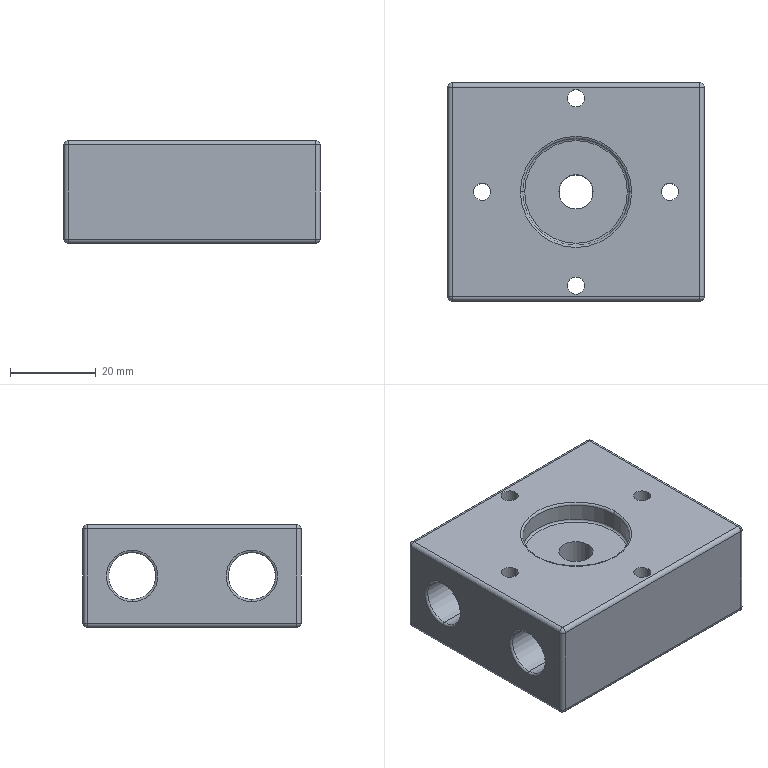Part | SolidWorks | features ICE 3, Fillet 2, Cut 1, Extrusion 1 | 1 solid | 55 faces | box 60 x 51 x 24 mm | volume 57298 mm3 | cylinder 28 | torus 12 | sphere 8 | plane 7 | commonest cylinder face diameters 2 x12 4 x8 11 x4 8 x2 25 x2
STEP:
#1=CARTESIAN_POINT('',(-19.92,0.,12.));
#2=VERTEX_POINT('',#1);
#3=CARTESIAN_POINT('',(-23.92,0.,12.));
#4=VERTEX_POINT('',#3);
#5=CARTESIAN_POINT('',(-21.92,0.,12.));
#6=DIRECTION('',(0.,0.,-1.));
#7=DIRECTION('',(-1.,0.,0.));
#8=AXIS2_PLACEMENT_3D('',#5,#6,#7);
#9=CIRCLE('',#8,2.);
#10=EDGE_CURVE('',#2,#4,#9,.T.);
#11=ORIENTED_EDGE('',*,*,#10,.F.);
#12=CARTESIAN_POINT('',(-19.92,0.,-12.));
#13=VERTEX_POINT('',#12);
#14=CARTESIAN_POINT('',(-19.92,0.,12.));
#15=DIRECTION('',(0.,0.,-1.));
#16=VECTOR('',#15,1000.);
#17=LINE('',#14,#16);
#18=EDGE_CURVE('',#2,#13,#17,.T.);
#19=ORIENTED_EDGE('',*,*,#18,.T.);
#20=CARTESIAN_POINT('',(-23.92,0.,-12.));
#21=VERTEX_POINT('',#20);
#22=CARTESIAN_POINT('',(-21.92,0.,-12.));
#23=DIRECTION('',(0.,0.,-1.));
#24=DIRECTION('',(-1.,0.,0.));
#25=AXIS2_PLACEMENT_3D('',#22,#23,#24);
#26=CIRCLE('',#25,2.);
#27=EDGE_CURVE('',#13,#21,#26,.T.);
#28=ORIENTED_EDGE('',*,*,#27,.T.);
#29=CARTESIAN_POINT('',(-23.92,0.,12.));
#30=DIRECTION('',(0.,0.,-1.));
#31=VECTOR('',#30,1000.);
#32=LINE('',#29,#31);
#33=EDGE_CURVE('',#4,#21,#32,.T.);
#34=ORIENTED_EDGE('',*,*,#33,.F.);
#35=EDGE_LOOP('',(#11,#19,#28,#34));
#36=FACE_OUTER_BOUND('',#35,.T.);
#37=CARTESIAN_POINT('',(-21.92,0.,12.));
#38=DIRECTION('',(0.,0.,-1.));
#39=DIRECTION('',(-1.,0.,0.));
#40=AXIS2_PLACEMENT_3D('',#37,#38,#39);
#41=CYLINDRICAL_SURFACE('',#40,2.);
#42=ADVANCED_FACE('',(#36),#41,.F.);
#43=CARTESIAN_POINT('',(2.,21.92,12.));
#44=VERTEX_POINT('',#43);
#45=CARTESIAN_POINT('',(-2.,21.92,12.));
#46=VERTEX_POINT('',#45);
#47=CARTESIAN_POINT('',(0.,21.92,12.));
#48=DIRECTION('',(0.,0.,-1.));
#49=DIRECTION('',(-1.,0.,0.));
#50=AXIS2_PLACEMENT_3D('',#47,#48,#49);
#51=CIRCLE('',#50,2.);
#52=EDGE_CURVE('',#44,#46,#51,.T.);
#53=ORIENTED_EDGE('',*,*,#52,.F.);
#54=CARTESIAN_POINT('',(2.,21.92,-12.));
#55=VERTEX_POINT('',#54);
#56=CARTESIAN_POINT('',(2.,21.92,12.));
#57=DIRECTION('',(0.,0.,-1.));
#58=VECTOR('',#57,1000.);
#59=LINE('',#56,#58);
#60=EDGE_CURVE('',#44,#55,#59,.T.);
#61=ORIENTED_EDGE('',*,*,#60,.T.);
#62=CARTESIAN_POINT('',(-2.,21.92,-12.));
#63=VERTEX_POINT('',#62);
#64=CARTESIAN_POINT('',(0.,21.92,-12.));
#65=DIRECTION('',(0.,0.,-1.));
#66=DIRECTION('',(-1.,0.,0.));
#67=AXIS2_PLACEMENT_3D('',#64,#65,#66);
#68=CIRCLE('',#67,2.);
#69=EDGE_CURVE('',#55,#63,#68,.T.);
#70=ORIENTED_EDGE('',*,*,#69,.T.);
#71=CARTESIAN_POINT('',(-2.,21.92,12.));
#72=DIRECTION('',(0.,0.,-1.));
#73=VECTOR('',#72,1000.);
#74=LINE('',#71,#73);
#75=EDGE_CURVE('',#46,#63,#74,.T.);
#76=ORIENTED_EDGE('',*,*,#75,.F.);
#77=EDGE_LOOP('',(#53,#61,#70,#76));
#78=FACE_OUTER_BOUND('',#77,.T.);
#79=CARTESIAN_POINT('',(0.,21.92,12.));
#80=DIRECTION('',(0.,0.,-1.));
#81=DIRECTION('',(-1.,0.,0.));
#82=AXIS2_PLACEMENT_3D('',#79,#80,#81);
#83=CYLINDRICAL_SURFACE('',#82,2.);
#84=ADVANCED_FACE('',(#78),#83,.F.);
#85=CARTESIAN_POINT('',(23.92,0.,12.));
#86=VERTEX_POINT('',#85);
#87=CARTESIAN_POINT('',(19.92,0.,12.));
#88=VERTEX_POINT('',#87);
#89=CARTESIAN_POINT('',(21.92,0.,12.));
#90=DIRECTION('',(0.,0.,-1.));
#91=DIRECTION('',(-1.,0.,0.));
#92=AXIS2_PLACEMENT_3D('',#89,#90,#91);
#93=CIRCLE('',#92,2.);
#94=EDGE_CURVE('',#86,#88,#93,.T.);
#95=ORIENTED_EDGE('',*,*,#94,.F.);
#96=CARTESIAN_POINT('',(23.92,0.,-12.));
#97=VERTEX_POINT('',#96);
#98=CARTESIAN_POINT('',(23.92,0.,12.));
#99=DIRECTION('',(0.,0.,-1.));
#100=VECTOR('',#99,1000.);
#101=LINE('',#98,#100);
#102=EDGE_CURVE('',#86,#97,#101,.T.);
#103=ORIENTED_EDGE('',*,*,#102,.T.);
#104=CARTESIAN_POINT('',(19.92,0.,-12.));
#105=VERTEX_POINT('',#104);
#106=CARTESIAN_POINT('',(21.92,0.,-12.));
#107=DIRECTION('',(0.,0.,-1.));
#108=DIRECTION('',(-1.,0.,0.));
#109=AXIS2_PLACEMENT_3D('',#106,#107,#108);
#110=CIRCLE('',#109,2.);
#111=EDGE_CURVE('',#97,#105,#110,.T.);
#112=ORIENTED_EDGE('',*,*,#111,.T.);
#113=CARTESIAN_POINT('',(19.92,0.,12.));
#114=DIRECTION('',(0.,0.,-1.));
#115=VECTOR('',#114,1000.);
#116=LINE('',#113,#115);
#117=EDGE_CURVE('',#88,#105,#116,.T.);
#118=ORIENTED_EDGE('',*,*,#117,.F.);
#119=EDGE_LOOP('',(#95,#103,#112,#118));
#120=FACE_OUTER_BOUND('',#119,.T.);
#121=CARTESIAN_POINT('',(21.92,0.,12.));
#122=DIRECTION('',(0.,0.,-1.));
#123=DIRECTION('',(-1.,0.,0.));
#124=AXIS2_PLACEMENT_3D('',#121,#122,#123);
#125=CYLINDRICAL_SURFACE('',#124,2.);
#126=ADVANCED_FACE('',(#120),#125,.F.);
#127=CARTESIAN_POINT('',(2.,-21.92,12.));
#128=VERTEX_POINT('',#127);
#129=CARTESIAN_POINT('',(-2.,-21.92,12.));
#130=VERTEX_POINT('',#129);
#131=CARTESIAN_POINT('',(0.,-21.92,12.));
#132=DIRECTION('',(0.,0.,-1.));
#133=DIRECTION('',(-1.,0.,0.));
#134=AXIS2_PLACEMENT_3D('',#131,#132,#133);
#135=CIRCLE('',#134,2.);
#136=EDGE_CURVE('',#128,#130,#135,.T.);
#137=ORIENTED_EDGE('',*,*,#136,.F.);
#138=CARTESIAN_POINT('',(2.,-21.92,-12.));
#139=VERTEX_POINT('',#138);
#140=CARTESIAN_POINT('',(2.,-21.92,12.));
#141=DIRECTION('',(0.,0.,-1.));
#142=VECTOR('',#141,1000.);
#143=LINE('',#140,#142);
#144=EDGE_CURVE('',#128,#139,#143,.T.);
#145=ORIENTED_EDGE('',*,*,#144,.T.);
#146=CARTESIAN_POINT('',(-2.,-21.92,-12.));
#147=VERTEX_POINT('',#146);
#148=CARTESIAN_POINT('',(0.,-21.92,-12.));
#149=DIRECTION('',(0.,0.,-1.));
#150=DIRECTION('',(-1.,0.,0.));
#151=AXIS2_PLACEMENT_3D('',#148,#149,#150);
#152=CIRCLE('',#151,2.);
#153=EDGE_CURVE('',#139,#147,#152,.T.);
#154=ORIENTED_EDGE('',*,*,#153,.T.);
#155=CARTESIAN_POINT('',(-2.,-21.92,12.));
#156=DIRECTION('',(0.,0.,-1.));
#157=VECTOR('',#156,1000.);
#158=LINE('',#155,#157);
#159=EDGE_CURVE('',#130,#147,#158,.T.);
#160=ORIENTED_EDGE('',*,*,#159,.F.);
#161=EDGE_LOOP('',(#137,#145,#154,#160));
#162=FACE_OUTER_BOUND('',#161,.T.);
#163=CARTESIAN_POINT('',(0.,-21.92,12.));
#164=DIRECTION('',(0.,0.,-1.));
#165=DIRECTION('',(-1.,0.,0.));
#166=AXIS2_PLACEMENT_3D('',#163,#164,#165);
#167=CYLINDRICAL_SURFACE('',#166,2.);
#168=ADVANCED_FACE('',(#162),#167,.F.);
#169=CARTESIAN_POINT('',(-4.,0.,7.));
#170=VERTEX_POINT('',#169);
#171=CARTESIAN_POINT('',(4.,0.,7.));
#172=VERTEX_POINT('',#171);
#173=CARTESIAN_POINT('',(0.,0.,7.));
#174=DIRECTION('',(0.,0.,1.));
#175=DIRECTION('',(1.,0.,0.));
#176=AXIS2_PLACEMENT_3D('',#173,#174,#175);
#177=CIRCLE('',#176,4.);
#178=EDGE_CURVE('',#170,#172,#177,.T.);
#179=ORIENTED_EDGE('',*,*,#178,.T.);
#180=CARTESIAN_POINT('',(4.,0.,-12.));
#181=VERTEX_POINT('',#180);
#182=CARTESIAN_POINT('',(4.,0.,12.));
#183=DIRECTION('',(0.,0.,-1.));
#184=VECTOR('',#183,1000.);
#185=LINE('',#182,#184);
#186=EDGE_CURVE('',#172,#181,#185,.T.);
#187=ORIENTED_EDGE('',*,*,#186,.T.);
#188=CARTESIAN_POINT('',(-4.,0.,-12.));
#189=VERTEX_POINT('',#188);
#190=CARTESIAN_POINT('',(0.,0.,-12.));
#191=DIRECTION('',(0.,0.,-1.));
#192=DIRECTION('',(-1.,0.,0.));
#193=AXIS2_PLACEMENT_3D('',#190,#191,#192);
#194=CIRCLE('',#193,4.);
#195=EDGE_CURVE('',#181,#189,#194,.T.);
#196=ORIENTED_EDGE('',*,*,#195,.T.);
#197=CARTESIAN_POINT('',(-4.,0.,12.));
#198=DIRECTION('',(0.,0.,-1.));
#199=VECTOR('',#198,1000.);
#200=LINE('',#197,#199);
#201=EDGE_CURVE('',#170,#189,#200,.T.);
#202=ORIENTED_EDGE('',*,*,#201,.F.);
#203=EDGE_LOOP('',(#179,#187,#196,#202));
#204=FACE_OUTER_BOUND('',#203,.T.);
#205=CARTESIAN_POINT('',(0.,0.,12.));
#206=DIRECTION('',(0.,0.,-1.));
#207=DIRECTION('',(-1.,0.,0.));
#208=AXIS2_PLACEMENT_3D('',#205,#206,#207);
#209=CYLINDRICAL_SURFACE('',#208,4.);
#210=ADVANCED_FACE('',(#204),#209,.F.);
#211=CARTESIAN_POINT('',(-29.5,14.,5.5));
#212=VERTEX_POINT('',#211);
#213=CARTESIAN_POINT('',(-29.5,14.,-5.5));
#214=VERTEX_POINT('',#213);
#215=CARTESIAN_POINT('',(-29.5,14.,0.));
#216=DIRECTION('',(-1.,0.,0.));
#217=DIRECTION('',(0.,0.,-1.));
#218=AXIS2_PLACEMENT_3D('',#215,#216,#217);
#219=CIRCLE('',#218,5.5);
#220=EDGE_CURVE('',#212,#214,#219,.T.);
#221=ORIENTED_EDGE('',*,*,#220,.F.);
#222=CARTESIAN_POINT('',(-30.,14.,6.));
#223=VERTEX_POINT('',#222);
#224=CARTESIAN_POINT('',(-29.5,14.,6.));
#225=DIRECTION('',(0.,1.,0.));
#226=DIRECTION('',(0.,0.,1.));
#227=AXIS2_PLACEMENT_3D('',#224,#225,#226);
#228=CIRCLE('',#227,0.5);
#229=EDGE_CURVE('',#212,#223,#228,.T.);
#230=ORIENTED_EDGE('',*,*,#229,.T.);
#231=CARTESIAN_POINT('',(-30.,14.,-6.));
#232=VERTEX_POINT('',#231);
#233=CARTESIAN_POINT('',(-30.,14.,0.));
#234=DIRECTION('',(1.,0.,0.));
#235=DIRECTION('',(0.,0.,-1.));
#236=AXIS2_PLACEMENT_3D('',#233,#234,#235);
#237=CIRCLE('',#236,6.);
#238=EDGE_CURVE('',#232,#223,#237,.T.);
#239=ORIENTED_EDGE('',*,*,#238,.F.);
#240=CARTESIAN_POINT('',(-29.5,14.,-6.));
#241=DIRECTION('',(0.,-1.,0.));
#242=DIRECTION('',(0.,0.,-1.));
#243=AXIS2_PLACEMENT_3D('',#240,#241,#242);
#244=CIRCLE('',#243,0.5);
#245=EDGE_CURVE('',#214,#232,#244,.T.);
#246=ORIENTED_EDGE('',*,*,#245,.F.);
#247=EDGE_LOOP('',(#221,#230,#239,#246));
#248=FACE_OUTER_BOUND('',#247,.T.);
#249=CARTESIAN_POINT('',(-29.5,14.,0.));
#250=DIRECTION('',(1.,0.,0.));
#251=DIRECTION('',(0.,0.,-1.));
#252=AXIS2_PLACEMENT_3D('',#249,#250,#251);
#253=TOROIDAL_SURFACE('',#252,6.,0.5);
#254=ADVANCED_FACE('',(#248),#253,.T.);
#255=CARTESIAN_POINT('',(29.5,14.,-5.5));
#256=VERTEX_POINT('',#255);
#257=CARTESIAN_POINT('',(29.5,14.,5.5));
#258=VERTEX_POINT('',#257);
#259=CARTESIAN_POINT('',(29.5,14.,0.));
#260=DIRECTION('',(1.,0.,0.));
#261=DIRECTION('',(0.,0.,1.));
#262=AXIS2_PLACEMENT_3D('',#259,#260,#261);
#263=CIRCLE('',#262,5.5);
#264=EDGE_CURVE('',#256,#258,#263,.T.);
#265=ORIENTED_EDGE('',*,*,#264,.F.);
#266=CARTESIAN_POINT('',(30.,14.,-6.));
#267=VERTEX_POINT('',#266);
#268=CARTESIAN_POINT('',(29.5,14.,-6.));
#269=DIRECTION('',(0.,1.,0.));
#270=DIRECTION('',(0.,0.,1.));
#271=AXIS2_PLACEMENT_3D('',#268,#269,#270);
#272=CIRCLE('',#271,0.5);
#273=EDGE_CURVE('',#256,#267,#272,.T.);
#274=ORIENTED_EDGE('',*,*,#273,.T.);
#275=CARTESIAN_POINT('',(30.,14.,6.));
#276=VERTEX_POINT('',#275);
#277=CARTESIAN_POINT('',(30.,14.,0.));
#278=DIRECTION('',(-1.,0.,0.));
#279=DIRECTION('',(0.,0.,1.));
#280=AXIS2_PLACEMENT_3D('',#277,#278,#279);
#281=CIRCLE('',#280,6.);
#282=EDGE_CURVE('',#276,#267,#281,.T.);
#283=ORIENTED_EDGE('',*,*,#282,.F.);
#284=CARTESIAN_POINT('',(29.5,14.,6.));
#285=DIRECTION('',(0.,-1.,0.));
#286=DIRECTION('',(0.,0.,-1.));
#287=AXIS2_PLACEMENT_3D('',#284,#285,#286);
#288=CIRCLE('',#287,0.5);
#289=EDGE_CURVE('',#258,#276,#288,.T.);
#290=ORIENTED_EDGE('',*,*,#289,.F.);
#291=EDGE_LOOP('',(#265,#274,#283,#290));
#292=FACE_OUTER_BOUND('',#291,.T.);
#293=CARTESIAN_POINT('',(29.5,14.,0.));
#294=DIRECTION('',(-1.,0.,0.));
#295=DIRECTION('',(0.,0.,1.));
#296=AXIS2_PLACEMENT_3D('',#293,#294,#295);
#297=TOROIDAL_SURFACE('',#296,6.,0.5);
#298=ADVANCED_FACE('',(#292),#297,.T.);
#299=CARTESIAN_POINT('',(-29.5,-14.,5.5));
#300=VERTEX_POINT('',#299);
#301=CARTESIAN_POINT('',(-29.5,-14.,-5.5));
#302=VERTEX_POINT('',#301);
#303=CARTESIAN_POINT('',(-29.5,-14.,0.));
#304=DIRECTION('',(-1.,0.,0.));
#305=DIRECTION('',(0.,0.,-1.));
#306=AXIS2_PLACEMENT_3D('',#303,#304,#305);
#307=CIRCLE('',#306,5.5);
#308=EDGE_CURVE('',#300,#302,#307,.T.);
#309=ORIENTED_EDGE('',*,*,#308,.F.);
#310=CARTESIAN_POINT('',(-30.,-14.,6.));
#311=VERTEX_POINT('',#310);
#312=CARTESIAN_POINT('',(-29.5,-14.,6.));
#313=DIRECTION('',(0.,1.,0.));
#314=DIRECTION('',(0.,0.,1.));
#315=AXIS2_PLACEMENT_3D('',#312,#313,#314);
#316=CIRCLE('',#315,0.5);
#317=EDGE_CURVE('',#300,#311,#316,.T.);
#318=ORIENTED_EDGE('',*,*,#317,.T.);
#319=CARTESIAN_POINT('',(-30.,-14.,-6.));
#320=VERTEX_POINT('',#319);
#321=CARTESIAN_POINT('',(-30.,-14.,0.));
#322=DIRECTION('',(1.,0.,0.));
#323=DIRECTION('',(0.,0.,-1.));
#324=AXIS2_PLACEMENT_3D('',#321,#322,#323);
#325=CIRCLE('',#324,6.);
#326=EDGE_CURVE('',#320,#311,#325,.T.);
#327=ORIENTED_EDGE('',*,*,#326,.F.);
#328=CARTESIAN_POINT('',(-29.5,-14.,-6.));
#329=DIRECTION('',(0.,-1.,0.));
#330=DIRECTION('',(0.,0.,-1.));
#331=AXIS2_PLACEMENT_3D('',#328,#329,#330);
#332=CIRCLE('',#331,0.5);
#333=EDGE_CURVE('',#302,#320,#332,.T.);
#334=ORIENTED_EDGE('',*,*,#333,.F.);
#335=EDGE_LOOP('',(#309,#318,#327,#334));
#336=FACE_OUTER_BOUND('',#335,.T.);
#337=CARTESIAN_POINT('',(-29.5,-14.,0.));
#338=DIRECTION('',(1.,0.,0.));
#339=DIRECTION('',(0.,0.,-1.));
#340=AXIS2_PLACEMENT_3D('',#337,#338,#339);
#341=TOROIDAL_SURFACE('',#340,6.,0.5);
#342=ADVANCED_FACE('',(#336),#341,.T.);
#343=CARTESIAN_POINT('',(29.5,-14.,-5.5));
#344=VERTEX_POINT('',#343);
#345=CARTESIAN_POINT('',(29.5,-14.,5.5));
#346=VERTEX_POINT('',#345);
#347=CARTESIAN_POINT('',(29.5,-14.,0.));
#348=DIRECTION('',(1.,0.,0.));
#349=DIRECTION('',(0.,0.,1.));
#350=AXIS2_PLACEMENT_3D('',#347,#348,#349);
#351=CIRCLE('',#350,5.5);
#352=EDGE_CURVE('',#344,#346,#351,.T.);
#353=ORIENTED_EDGE('',*,*,#352,.F.);
#354=CARTESIAN_POINT('',(30.,-14.,-6.));
#355=VERTEX_POINT('',#354);
#356=CARTESIAN_POINT('',(29.5,-14.,-6.));
#357=DIRECTION('',(0.,1.,0.));
#358=DIRECTION('',(0.,0.,1.));
#359=AXIS2_PLACEMENT_3D('',#356,#357,#358);
#360=CIRCLE('',#359,0.5);
#361=EDGE_CURVE('',#344,#355,#360,.T.);
#362=ORIENTED_EDGE('',*,*,#361,.T.);
#363=CARTESIAN_POINT('',(30.,-14.,6.));
#364=VERTEX_POINT('',#363);
#365=CARTESIAN_POINT('',(30.,-14.,0.));
#366=DIRECTION('',(-1.,0.,0.));
#367=DIRECTION('',(0.,0.,1.));
#368=AXIS2_PLACEMENT_3D('',#365,#366,#367);
#369=CIRCLE('',#368,6.);
#370=EDGE_CURVE('',#364,#355,#369,.T.);
#371=ORIENTED_EDGE('',*,*,#370,.F.);
#372=CARTESIAN_POINT('',(29.5,-14.,6.));
#373=DIRECTION('',(0.,-1.,0.));
#374=DIRECTION('',(0.,0.,-1.));
#375=AXIS2_PLACEMENT_3D('',#372,#373,#374);
#376=CIRCLE('',#375,0.5);
#377=EDGE_CURVE('',#346,#364,#376,.T.);
#378=ORIENTED_EDGE('',*,*,#377,.F.);
#379=EDGE_LOOP('',(#353,#362,#371,#378));
#380=FACE_OUTER_BOUND('',#379,.T.);
#381=CARTESIAN_POINT('',(29.5,-14.,0.));
#382=DIRECTION('',(-1.,0.,0.));
#383=DIRECTION('',(0.,0.,1.));
#384=AXIS2_PLACEMENT_3D('',#381,#382,#383);
#385=TOROIDAL_SURFACE('',#384,6.,0.5);
#386=ADVANCED_FACE('',(#380),#385,.T.);
#387=CARTESIAN_POINT('',(-12.,0.,7.));
#388=VERTEX_POINT('',#387);
#389=CARTESIAN_POINT('',(12.,0.,7.));
#390=VERTEX_POINT('',#389);
#391=CARTESIAN_POINT('',(0.,0.,7.));
#392=DIRECTION('',(0.,0.,1.));
#393=DIRECTION('',(1.,0.,0.));
#394=AXIS2_PLACEMENT_3D('',#391,#392,#393);
#395=CIRCLE('',#394,12.);
#396=EDGE_CURVE('',#388,#390,#395,.T.);
#397=ORIENTED_EDGE('',*,*,#396,.F.);
#398=CARTESIAN_POINT('',(-12.5,0.,7.5));
#399=VERTEX_POINT('',#398);
#400=CARTESIAN_POINT('',(-12.,0.,7.5));
#401=DIRECTION('',(0.,1.,0.));
#402=DIRECTION('',(-1.,0.,0.));
#403=AXIS2_PLACEMENT_3D('',#400,#401,#402);
#404=CIRCLE('',#403,0.5);
#405=EDGE_CURVE('',#388,#399,#404,.T.);
#406=ORIENTED_EDGE('',*,*,#405,.T.);
#407=CARTESIAN_POINT('',(12.5,0.,7.5));
#408=VERTEX_POINT('',#407);
#409=CARTESIAN_POINT('',(0.,0.,7.5));
#410=DIRECTION('',(0.,0.,-1.));
#411=DIRECTION('',(1.,0.,0.));
#412=AXIS2_PLACEMENT_3D('',#409,#410,#411);
#413=CIRCLE('',#412,12.5);
#414=EDGE_CURVE('',#408,#399,#413,.T.);
#415=ORIENTED_EDGE('',*,*,#414,.F.);
#416=CARTESIAN_POINT('',(12.,0.,7.5));
#417=DIRECTION('',(0.,-1.,0.));
#418=DIRECTION('',(0.,0.,-1.));
#419=AXIS2_PLACEMENT_3D('',#416,#417,#418);
#420=CIRCLE('',#419,0.5);
#421=EDGE_CURVE('',#390,#408,#420,.T.);
#422=ORIENTED_EDGE('',*,*,#421,.F.);
#423=EDGE_LOOP('',(#397,#406,#415,#422));
#424=FACE_OUTER_BOUND('',#423,.T.);
#425=CARTESIAN_POINT('',(0.,0.,7.5));
#426=DIRECTION('',(0.,0.,1.));
#427=DIRECTION('',(1.,0.,0.));
#428=AXIS2_PLACEMENT_3D('',#425,#426,#427);
#429=TOROIDAL_SURFACE('',#428,12.,0.5);
#430=ADVANCED_FACE('',(#424),#429,.F.);
#431=CARTESIAN_POINT('',(-13.,0.,12.));
#432=VERTEX_POINT('',#431);
#433=CARTESIAN_POINT('',(13.,0.,12.));
#434=VERTEX_POINT('',#433);
#435=CARTESIAN_POINT('',(0.,0.,12.));
#436=DIRECTION('',(0.,0.,-1.));
#437=DIRECTION('',(1.,0.,0.));
#438=AXIS2_PLACEMENT_3D('',#435,#436,#437);
#439=CIRCLE('',#438,13.);
#440=EDGE_CURVE('',#432,#434,#439,.T.);
#441=ORIENTED_EDGE('',*,*,#440,.F.);
#442=CARTESIAN_POINT('',(-12.5,0.,11.5));
#443=VERTEX_POINT('',#442);
#444=CARTESIAN_POINT('',(-13.,0.,11.5));
#445=DIRECTION('',(0.,1.,0.));
#446=DIRECTION('',(-1.,0.,0.));
#447=AXIS2_PLACEMENT_3D('',#444,#445,#446);
#448=CIRCLE('',#447,0.5);
#449=EDGE_CURVE('',#432,#443,#448,.T.);
#450=ORIENTED_EDGE('',*,*,#449,.T.);
#451=CARTESIAN_POINT('',(12.5,0.,11.5));
#452=VERTEX_POINT('',#451);
#453=CARTESIAN_POINT('',(0.,0.,11.5));
#454=DIRECTION('',(0.,0.,1.));
#455=DIRECTION('',(1.,0.,0.));
#456=AXIS2_PLACEMENT_3D('',#453,#454,#455);
#457=CIRCLE('',#456,12.5);
#458=EDGE_CURVE('',#452,#443,#457,.T.);
#459=ORIENTED_EDGE('',*,*,#458,.F.);
#460=CARTESIAN_POINT('',(13.,0.,11.5));
#461=DIRECTION('',(0.,-1.,0.));
#462=DIRECTION('',(0.,0.,-1.));
#463=AXIS2_PLACEMENT_3D('',#460,#461,#462);
#464=CIRCLE('',#463,0.5);
#465=EDGE_CURVE('',#434,#452,#464,.T.);
#466=ORIENTED_EDGE('',*,*,#465,.F.);
#467=EDGE_LOOP('',(#441,#450,#459,#466));
#468=FACE_OUTER_BOUND('',#467,.T.);
#469=CARTESIAN_POINT('',(0.,0.,11.5));
#470=DIRECTION('',(0.,0.,1.));
#471=DIRECTION('',(1.,0.,0.));
#472=AXIS2_PLACEMENT_3D('',#469,#470,#471);
#473=TOROIDAL_SURFACE('',#472,13.,0.5);
#474=ADVANCED_FACE('',(#468),#473,.T.);
#475=CARTESIAN_POINT('',(-29.5,-14.,0.));
#476=DIRECTION('',(-1.,0.,0.));
#477=DIRECTION('',(0.,0.,-1.));
#478=AXIS2_PLACEMENT_3D('',#475,#476,#477);
#479=CIRCLE('',#478,5.5);
#480=EDGE_CURVE('',#302,#300,#479,.T.);
#481=ORIENTED_EDGE('',*,*,#480,.T.);
#482=CARTESIAN_POINT('',(-30.,-14.,5.5));
#483=DIRECTION('',(1.,0.,0.));
#484=VECTOR('',#483,1000.);
#485=LINE('',#482,#484);
#486=EDGE_CURVE('',#300,#346,#485,.T.);
#487=ORIENTED_EDGE('',*,*,#486,.T.);
#488=CARTESIAN_POINT('',(29.5,-14.,0.));
#489=DIRECTION('',(1.,0.,0.));
#490=DIRECTION('',(0.,0.,1.));
#491=AXIS2_PLACEMENT_3D('',#488,#489,#490);
#492=CIRCLE('',#491,5.5);
#493=EDGE_CURVE('',#346,#344,#492,.T.);
#494=ORIENTED_EDGE('',*,*,#493,.T.);
#495=CARTESIAN_POINT('',(-30.,-14.,-5.5));
#496=DIRECTION('',(1.,0.,0.));
#497=VECTOR('',#496,1000.);
#498=LINE('',#495,#497);
#499=EDGE_CURVE('',#302,#344,#498,.T.);
#500=ORIENTED_EDGE('',*,*,#499,.F.);
#501=EDGE_LOOP('',(#481,#487,#494,#500));
#502=FACE_OUTER_BOUND('',#501,.T.);
#503=CARTESIAN_POINT('',(-30.,-14.,0.));
#504=DIRECTION('',(1.,0.,0.));
#505=DIRECTION('',(0.,0.,-1.));
#506=AXIS2_PLACEMENT_3D('',#503,#504,#505);
#507=CYLINDRICAL_SURFACE('',#506,5.5);
#508=ADVANCED_FACE('',(#502),#507,.F.);
#509=CARTESIAN_POINT('',(-29.5,14.,0.));
#510=DIRECTION('',(-1.,0.,0.));
#511=DIRECTION('',(0.,0.,-1.));
#512=AXIS2_PLACEMENT_3D('',#509,#510,#511);
#513=CIRCLE('',#512,5.5);
#514=EDGE_CURVE('',#214,#212,#513,.T.);
#515=ORIENTED_EDGE('',*,*,#514,.T.);
#516=CARTESIAN_POINT('',(-30.,14.,5.5));
#517=DIRECTION('',(1.,0.,0.));
#518=VECTOR('',#517,1000.);
#519=LINE('',#516,#518);
#520=EDGE_CURVE('',#212,#258,#519,.T.);
#521=ORIENTED_EDGE('',*,*,#520,.T.);
#522=CARTESIAN_POINT('',(29.5,14.,0.));
#523=DIRECTION('',(1.,0.,0.));
#524=DIRECTION('',(0.,0.,1.));
#525=AXIS2_PLACEMENT_3D('',#522,#523,#524);
#526=CIRCLE('',#525,5.5);
#527=EDGE_CURVE('',#258,#256,#526,.T.);
#528=ORIENTED_EDGE('',*,*,#527,.T.);
#529=CARTESIAN_POINT('',(-30.,14.,-5.5));
#530=DIRECTION('',(1.,0.,0.));
#531=VECTOR('',#530,1000.);
#532=LINE('',#529,#531);
#533=EDGE_CURVE('',#214,#256,#532,.T.);
#534=ORIENTED_EDGE('',*,*,#533,.F.);
#535=EDGE_LOOP('',(#515,#521,#528,#534));
#536=FACE_OUTER_BOUND('',#535,.T.);
#537=CARTESIAN_POINT('',(-30.,14.,0.));
#538=DIRECTION('',(1.,0.,0.));
#539=DIRECTION('',(0.,0.,-1.));
#540=AXIS2_PLACEMENT_3D('',#537,#538,#539);
#541=CYLINDRICAL_SURFACE('',#540,5.5);
#542=ADVANCED_FACE('',(#536),#541,.F.);
#543=ORIENTED_EDGE('',*,*,#414,.T.);
#544=CARTESIAN_POINT('',(-12.5,0.,7.));
#545=DIRECTION('',(0.,0.,1.));
#546=VECTOR('',#545,1000.);
#547=LINE('',#544,#546);
#548=EDGE_CURVE('',#399,#443,#547,.T.);
#549=ORIENTED_EDGE('',*,*,#548,.T.);
#550=CARTESIAN_POINT('',(0.,0.,11.5));
#551=DIRECTION('',(0.,0.,1.));
#552=DIRECTION('',(1.,0.,0.));
#553=AXIS2_PLACEMENT_3D('',#550,#551,#552);
#554=CIRCLE('',#553,12.5);
#555=EDGE_CURVE('',#443,#452,#554,.T.);
#556=ORIENTED_EDGE('',*,*,#555,.T.);
#557=CARTESIAN_POINT('',(12.5,0.,7.));
#558=DIRECTION('',(0.,0.,1.));
#559=VECTOR('',#558,1000.);
#560=LINE('',#557,#559);
#561=EDGE_CURVE('',#408,#452,#560,.T.);
#562=ORIENTED_EDGE('',*,*,#561,.F.);
#563=EDGE_LOOP('',(#543,#549,#556,#562));
#564=FACE_OUTER_BOUND('',#563,.T.);
#565=CARTESIAN_POINT('',(0.,0.,7.));
#566=DIRECTION('',(0.,0.,1.));
#567=DIRECTION('',(1.,0.,0.));
#568=AXIS2_PLACEMENT_3D('',#565,#566,#567);
#569=CYLINDRICAL_SURFACE('',#568,12.5);
#570=ADVANCED_FACE('',(#564),#569,.F.);
#571=ORIENTED_EDGE('',*,*,#326,.T.);
#572=CARTESIAN_POINT('',(-30.,-14.,0.));
#573=DIRECTION('',(1.,0.,0.));
#574=DIRECTION('',(0.,0.,-1.));
#575=AXIS2_PLACEMENT_3D('',#572,#573,#574);
#576=CIRCLE('',#575,6.);
#577=EDGE_CURVE('',#311,#320,#576,.T.);
#578=ORIENTED_EDGE('',*,*,#577,.T.);
#579=EDGE_LOOP('',(#571,#578));
#580=FACE_BOUND('',#579,.T.);
#581=ORIENTED_EDGE('',*,*,#238,.T.);
#582=CARTESIAN_POINT('',(-30.,14.,0.));
#583=DIRECTION('',(1.,0.,0.));
#584=DIRECTION('',(0.,0.,-1.));
#585=AXIS2_PLACEMENT_3D('',#582,#583,#584);
#586=CIRCLE('',#585,6.);
#587=EDGE_CURVE('',#223,#232,#586,.T.);
#588=ORIENTED_EDGE('',*,*,#587,.T.);
#589=EDGE_LOOP('',(#581,#588));
#590=FACE_BOUND('',#589,.T.);
#591=CARTESIAN_POINT('',(-30.,24.5,11.));
#592=VERTEX_POINT('',#591);
#593=CARTESIAN_POINT('',(-30.,24.5,-11.));
#594=VERTEX_POINT('',#593);
#595=CARTESIAN_POINT('',(-30.,24.5,12.));
#596=DIRECTION('',(0.,0.,-1.));
#597=VECTOR('',#596,1000.);
#598=LINE('',#595,#597);
#599=EDGE_CURVE('',#592,#594,#598,.T.);
#600=ORIENTED_EDGE('',*,*,#599,.T.);
#601=CARTESIAN_POINT('',(-30.,-24.5,-11.));
#602=VERTEX_POINT('',#601);
#603=CARTESIAN_POINT('',(-30.,-25.5,-11.));
#604=DIRECTION('',(0.,-1.,0.));
#605=VECTOR('',#604,1000.);
#606=LINE('',#603,#605);
#607=EDGE_CURVE('',#594,#602,#606,.T.);
#608=ORIENTED_EDGE('',*,*,#607,.T.);
#609=CARTESIAN_POINT('',(-30.,-24.5,11.));
#610=VERTEX_POINT('',#609);
#611=CARTESIAN_POINT('',(-30.,-24.5,12.));
#612=DIRECTION('',(0.,0.,1.));
#613=VECTOR('',#612,1000.);
#614=LINE('',#611,#613);
#615=EDGE_CURVE('',#602,#610,#614,.T.);
#616=ORIENTED_EDGE('',*,*,#615,.T.);
#617=CARTESIAN_POINT('',(-30.,25.5,11.));
#618=DIRECTION('',(0.,1.,0.));
#619=VECTOR('',#618,1000.);
#620=LINE('',#617,#619);
#621=EDGE_CURVE('',#610,#592,#620,.T.);
#622=ORIENTED_EDGE('',*,*,#621,.T.);
#623=EDGE_LOOP('',(#600,#608,#616,#622));
#624=FACE_OUTER_BOUND('',#623,.T.);
#625=CARTESIAN_POINT('',(-30.,-25.5,12.));
#626=DIRECTION('',(1.,0.,0.));
#627=DIRECTION('',(0.,0.,-1.));
#628=AXIS2_PLACEMENT_3D('',#625,#626,#627);
#629=PLANE('',#628);
#630=ADVANCED_FACE('',(#580,#590,#624),#629,.F.);
#631=CARTESIAN_POINT('',(29.,-25.5,11.));
#632=VERTEX_POINT('',#631);
#633=CARTESIAN_POINT('',(-29.,-25.5,11.));
#634=VERTEX_POINT('',#633);
#635=CARTESIAN_POINT('',(-30.,-25.5,11.));
#636=DIRECTION('',(-1.,0.,0.));
#637=VECTOR('',#636,1000.);
#638=LINE('',#635,#637);
#639=EDGE_CURVE('',#632,#634,#638,.T.);
#640=ORIENTED_EDGE('',*,*,#639,.T.);
#641=CARTESIAN_POINT('',(-29.,-25.5,-11.));
#642=VERTEX_POINT('',#641);
#643=CARTESIAN_POINT('',(-29.,-25.5,12.));
#644=DIRECTION('',(0.,0.,-1.));
#645=VECTOR('',#644,1000.);
#646=LINE('',#643,#645);
#647=EDGE_CURVE('',#634,#642,#646,.T.);
#648=ORIENTED_EDGE('',*,*,#647,.T.);
#649=CARTESIAN_POINT('',(29.,-25.5,-11.));
#650=VERTEX_POINT('',#649);
#651=CARTESIAN_POINT('',(30.,-25.5,-11.));
#652=DIRECTION('',(1.,0.,0.));
#653=VECTOR('',#652,1000.);
#654=LINE('',#651,#653);
#655=EDGE_CURVE('',#642,#650,#654,.T.);
#656=ORIENTED_EDGE('',*,*,#655,.T.);
#657=CARTESIAN_POINT('',(29.,-25.5,12.));
#658=DIRECTION('',(0.,0.,1.));
#659=VECTOR('',#658,1000.);
#660=LINE('',#657,#659);
#661=EDGE_CURVE('',#650,#632,#660,.T.);
#662=ORIENTED_EDGE('',*,*,#661,.T.);
#663=EDGE_LOOP('',(#640,#648,#656,#662));
#664=FACE_OUTER_BOUND('',#663,.T.);
#665=CARTESIAN_POINT('',(30.,-25.5,12.));
#666=DIRECTION('',(0.,1.,0.));
#667=DIRECTION('',(-1.,0.,0.));
#668=AXIS2_PLACEMENT_3D('',#665,#666,#667);
#669=PLANE('',#668);
#670=ADVANCED_FACE('',(#664),#669,.F.);
#671=ORIENTED_EDGE('',*,*,#370,.T.);
#672=CARTESIAN_POINT('',(30.,-14.,0.));
#673=DIRECTION('',(-1.,0.,0.));
#674=DIRECTION('',(0.,0.,1.));
#675=AXIS2_PLACEMENT_3D('',#672,#673,#674);
#676=CIRCLE('',#675,6.);
#677=EDGE_CURVE('',#355,#364,#676,.T.);
#678=ORIENTED_EDGE('',*,*,#677,.T.);
#679=EDGE_LOOP('',(#671,#678));
#680=FACE_BOUND('',#679,.T.);
#681=ORIENTED_EDGE('',*,*,#282,.T.);
#682=CARTESIAN_POINT('',(30.,14.,0.));
#683=DIRECTION('',(-1.,0.,0.));
#684=DIRECTION('',(0.,0.,1.));
#685=AXIS2_PLACEMENT_3D('',#682,#683,#684);
#686=CIRCLE('',#685,6.);
#687=EDGE_CURVE('',#267,#276,#686,.T.);
#688=ORIENTED_EDGE('',*,*,#687,.T.);
#689=EDGE_LOOP('',(#681,#688));
#690=FACE_BOUND('',#689,.T.);
#691=CARTESIAN_POINT('',(30.,-24.5,11.));
#692=VERTEX_POINT('',#691);
#693=CARTESIAN_POINT('',(30.,-24.5,-11.));
#694=VERTEX_POINT('',#693);
#695=CARTESIAN_POINT('',(30.,-24.5,12.));
#696=DIRECTION('',(0.,0.,-1.));
#697=VECTOR('',#696,1000.);
#698=LINE('',#695,#697);
#699=EDGE_CURVE('',#692,#694,#698,.T.);
#700=ORIENTED_EDGE('',*,*,#699,.T.);
#701=CARTESIAN_POINT('',(30.,24.5,-11.));
#702=VERTEX_POINT('',#701);
#703=CARTESIAN_POINT('',(30.,-25.5,-11.));
#704=DIRECTION('',(0.,1.,0.));
#705=VECTOR('',#704,1000.);
#706=LINE('',#703,#705);
#707=EDGE_CURVE('',#694,#702,#706,.T.);
#708=ORIENTED_EDGE('',*,*,#707,.T.);
#709=CARTESIAN_POINT('',(30.,24.5,11.));
#710=VERTEX_POINT('',#709);
#711=CARTESIAN_POINT('',(30.,24.5,12.));
#712=DIRECTION('',(0.,0.,1.));
#713=VECTOR('',#712,1000.);
#714=LINE('',#711,#713);
#715=EDGE_CURVE('',#702,#710,#714,.T.);
#716=ORIENTED_EDGE('',*,*,#715,.T.);
#717=CARTESIAN_POINT('',(30.,-25.5,11.));
#718=DIRECTION('',(0.,-1.,0.));
#719=VECTOR('',#718,1000.);
#720=LINE('',#717,#719);
#721=EDGE_CURVE('',#710,#692,#720,.T.);
#722=ORIENTED_EDGE('',*,*,#721,.T.);
#723=EDGE_LOOP('',(#700,#708,#716,#722));
#724=FACE_OUTER_BOUND('',#723,.T.);
#725=CARTESIAN_POINT('',(30.,-25.5,12.));
#726=DIRECTION('',(-1.,0.,0.));
#727=DIRECTION('',(0.,0.,1.));
#728=AXIS2_PLACEMENT_3D('',#725,#726,#727);
#729=PLANE('',#728);
#730=ADVANCED_FACE('',(#680,#690,#724),#729,.F.);
#731=CARTESIAN_POINT('',(-29.,25.5,11.));
#732=VERTEX_POINT('',#731);
#733=CARTESIAN_POINT('',(29.,25.5,11.));
#734=VERTEX_POINT('',#733);
#735=CARTESIAN_POINT('',(30.,25.5,11.));
#736=DIRECTION('',(1.,0.,0.));
#737=VECTOR('',#736,1000.);
#738=LINE('',#735,#737);
#739=EDGE_CURVE('',#732,#734,#738,.T.);
#740=ORIENTED_EDGE('',*,*,#739,.T.);
#741=CARTESIAN_POINT('',(29.,25.5,-11.));
#742=VERTEX_POINT('',#741);
#743=CARTESIAN_POINT('',(29.,25.5,12.));
#744=DIRECTION('',(0.,0.,-1.));
#745=VECTOR('',#744,1000.);
#746=LINE('',#743,#745);
#747=EDGE_CURVE('',#734,#742,#746,.T.);
#748=ORIENTED_EDGE('',*,*,#747,.T.);
#749=CARTESIAN_POINT('',(-29.,25.5,-11.));
#750=VERTEX_POINT('',#749);
#751=CARTESIAN_POINT('',(30.,25.5,-11.));
#752=DIRECTION('',(-1.,0.,0.));
#753=VECTOR('',#752,1000.);
#754=LINE('',#751,#753);
#755=EDGE_CURVE('',#742,#750,#754,.T.);
#756=ORIENTED_EDGE('',*,*,#755,.T.);
#757=CARTESIAN_POINT('',(-29.,25.5,12.));
#758=DIRECTION('',(0.,0.,1.));
#759=VECTOR('',#758,1000.);
#760=LINE('',#757,#759);
#761=EDGE_CURVE('',#750,#732,#760,.T.);
#762=ORIENTED_EDGE('',*,*,#761,.T.);
#763=EDGE_LOOP('',(#740,#748,#756,#762));
#764=FACE_OUTER_BOUND('',#763,.T.);
#765=CARTESIAN_POINT('',(30.,25.5,12.));
#766=DIRECTION('',(0.,-1.,0.));
#767=DIRECTION('',(1.,0.,0.));
#768=AXIS2_PLACEMENT_3D('',#765,#766,#767);
#769=PLANE('',#768);
#770=ADVANCED_FACE('',(#764),#769,.F.);
#771=CARTESIAN_POINT('',(-21.92,0.,12.));
#772=DIRECTION('',(0.,0.,-1.));
#773=DIRECTION('',(-1.,0.,0.));
#774=AXIS2_PLACEMENT_3D('',#771,#772,#773);
#775=CIRCLE('',#774,2.);
#776=EDGE_CURVE('',#4,#2,#775,.T.);
#777=ORIENTED_EDGE('',*,*,#776,.T.);
#778=ORIENTED_EDGE('',*,*,#10,.T.);
#779=EDGE_LOOP('',(#777,#778));
#780=FACE_BOUND('',#779,.T.);
#781=CARTESIAN_POINT('',(0.,21.92,12.));
#782=DIRECTION('',(0.,0.,-1.));
#783=DIRECTION('',(-1.,0.,0.));
#784=AXIS2_PLACEMENT_3D('',#781,#782,#783);
#785=CIRCLE('',#784,2.);
#786=EDGE_CURVE('',#46,#44,#785,.T.);
#787=ORIENTED_EDGE('',*,*,#786,.T.);
#788=ORIENTED_EDGE('',*,*,#52,.T.);
#789=EDGE_LOOP('',(#787,#788));
#790=FACE_BOUND('',#789,.T.);
#791=CARTESIAN_POINT('',(21.92,0.,12.));
#792=DIRECTION('',(0.,0.,-1.));
#793=DIRECTION('',(-1.,0.,0.));
#794=AXIS2_PLACEMENT_3D('',#791,#792,#793);
#795=CIRCLE('',#794,2.);
#796=EDGE_CURVE('',#88,#86,#795,.T.);
#797=ORIENTED_EDGE('',*,*,#796,.T.);
#798=ORIENTED_EDGE('',*,*,#94,.T.);
#799=EDGE_LOOP('',(#797,#798));
#800=FACE_BOUND('',#799,.T.);
#801=CARTESIAN_POINT('',(0.,-21.92,12.));
#802=DIRECTION('',(0.,0.,-1.));
#803=DIRECTION('',(-1.,0.,0.));
#804=AXIS2_PLACEMENT_3D('',#801,#802,#803);
#805=CIRCLE('',#804,2.);
#806=EDGE_CURVE('',#130,#128,#805,.T.);
#807=ORIENTED_EDGE('',*,*,#806,.T.);
#808=ORIENTED_EDGE('',*,*,#136,.T.);
#809=EDGE_LOOP('',(#807,#808));
#810=FACE_BOUND('',#809,.T.);
#811=CARTESIAN_POINT('',(0.,0.,12.));
#812=DIRECTION('',(0.,0.,-1.));
#813=DIRECTION('',(1.,0.,0.));
#814=AXIS2_PLACEMENT_3D('',#811,#812,#813);
#815=CIRCLE('',#814,13.);
#816=EDGE_CURVE('',#434,#432,#815,.T.);
#817=ORIENTED_EDGE('',*,*,#816,.T.);
#818=ORIENTED_EDGE('',*,*,#440,.T.);
#819=EDGE_LOOP('',(#817,#818));
#820=FACE_BOUND('',#819,.T.);
#821=CARTESIAN_POINT('',(29.,24.5,12.));
#822=VERTEX_POINT('',#821);
#823=CARTESIAN_POINT('',(-29.,24.5,12.));
#824=VERTEX_POINT('',#823);
#825=CARTESIAN_POINT('',(-30.,24.5,12.));
#826=DIRECTION('',(-1.,0.,0.));
#827=VECTOR('',#826,1000.);
#828=LINE('',#825,#827);
#829=EDGE_CURVE('',#822,#824,#828,.T.);
#830=ORIENTED_EDGE('',*,*,#829,.T.);
#831=CARTESIAN_POINT('',(-29.,-24.5,12.));
#832=VERTEX_POINT('',#831);
#833=CARTESIAN_POINT('',(-29.,-25.5,12.));
#834=DIRECTION('',(0.,-1.,0.));
#835=VECTOR('',#834,1000.);
#836=LINE('',#833,#835);
#837=EDGE_CURVE('',#824,#832,#836,.T.);
#838=ORIENTED_EDGE('',*,*,#837,.T.);
#839=CARTESIAN_POINT('',(29.,-24.5,12.));
#840=VERTEX_POINT('',#839);
#841=CARTESIAN_POINT('',(30.,-24.5,12.));
#842=DIRECTION('',(1.,0.,0.));
#843=VECTOR('',#842,1000.);
#844=LINE('',#841,#843);
#845=EDGE_CURVE('',#832,#840,#844,.T.);
#846=ORIENTED_EDGE('',*,*,#845,.T.);
#847=CARTESIAN_POINT('',(29.,25.5,12.));
#848=DIRECTION('',(0.,1.,0.));
#849=VECTOR('',#848,1000.);
#850=LINE('',#847,#849);
#851=EDGE_CURVE('',#840,#822,#850,.T.);
#852=ORIENTED_EDGE('',*,*,#851,.T.);
#853=EDGE_LOOP('',(#830,#838,#846,#852));
#854=FACE_OUTER_BOUND('',#853,.T.);
#855=CARTESIAN_POINT('',(0.,0.,12.));
#856=DIRECTION('',(0.,0.,1.));
#857=DIRECTION('',(1.,0.,0.));
#858=AXIS2_PLACEMENT_3D('',#855,#856,#857);
#859=PLANE('',#858);
#860=ADVANCED_FACE('',(#780,#790,#800,#810,#820,#854),#859,.T.);
#861=CARTESIAN_POINT('',(-21.92,0.,-12.));
#862=DIRECTION('',(0.,0.,-1.));
#863=DIRECTION('',(-1.,0.,0.));
#864=AXIS2_PLACEMENT_3D('',#861,#862,#863);
#865=CIRCLE('',#864,2.);
#866=EDGE_CURVE('',#21,#13,#865,.T.);
#867=ORIENTED_EDGE('',*,*,#866,.F.);
#868=ORIENTED_EDGE('',*,*,#27,.F.);
#869=EDGE_LOOP('',(#867,#868));
#870=FACE_BOUND('',#869,.T.);
#871=CARTESIAN_POINT('',(0.,21.92,-12.));
#872=DIRECTION('',(0.,0.,-1.));
#873=DIRECTION('',(-1.,0.,0.));
#874=AXIS2_PLACEMENT_3D('',#871,#872,#873);
#875=CIRCLE('',#874,2.);
#876=EDGE_CURVE('',#63,#55,#875,.T.);
#877=ORIENTED_EDGE('',*,*,#876,.F.);
#878=ORIENTED_EDGE('',*,*,#69,.F.);
#879=EDGE_LOOP('',(#877,#878));
#880=FACE_BOUND('',#879,.T.);
#881=CARTESIAN_POINT('',(21.92,0.,-12.));
#882=DIRECTION('',(0.,0.,-1.));
#883=DIRECTION('',(-1.,0.,0.));
#884=AXIS2_PLACEMENT_3D('',#881,#882,#883);
#885=CIRCLE('',#884,2.);
#886=EDGE_CURVE('',#105,#97,#885,.T.);
#887=ORIENTED_EDGE('',*,*,#886,.F.);
#888=ORIENTED_EDGE('',*,*,#111,.F.);
#889=EDGE_LOOP('',(#887,#888));
#890=FACE_BOUND('',#889,.T.);
#891=CARTESIAN_POINT('',(0.,-21.92,-12.));
#892=DIRECTION('',(0.,0.,-1.));
#893=DIRECTION('',(-1.,0.,0.));
#894=AXIS2_PLACEMENT_3D('',#891,#892,#893);
#895=CIRCLE('',#894,2.);
#896=EDGE_CURVE('',#147,#139,#895,.T.);
#897=ORIENTED_EDGE('',*,*,#896,.F.);
#898=ORIENTED_EDGE('',*,*,#153,.F.);
#899=EDGE_LOOP('',(#897,#898));
#900=FACE_BOUND('',#899,.T.);
#901=CARTESIAN_POINT('',(0.,0.,-12.));
#902=DIRECTION('',(0.,0.,-1.));
#903=DIRECTION('',(-1.,0.,0.));
#904=AXIS2_PLACEMENT_3D('',#901,#902,#903);
#905=CIRCLE('',#904,4.);
#906=EDGE_CURVE('',#189,#181,#905,.T.);
#907=ORIENTED_EDGE('',*,*,#906,.F.);
#908=ORIENTED_EDGE('',*,*,#195,.F.);
#909=EDGE_LOOP('',(#907,#908));
#910=FACE_BOUND('',#909,.T.);
#911=CARTESIAN_POINT('',(29.,-24.5,-12.));
#912=VERTEX_POINT('',#911);
#913=CARTESIAN_POINT('',(-29.,-24.5,-12.));
#914=VERTEX_POINT('',#913);
#915=CARTESIAN_POINT('',(0.,-24.5,-12.));
#916=DIRECTION('',(-1.,0.,0.));
#917=VECTOR('',#916,1000.);
#918=LINE('',#915,#917);
#919=EDGE_CURVE('',#912,#914,#918,.T.);
#920=ORIENTED_EDGE('',*,*,#919,.T.);
#921=CARTESIAN_POINT('',(-29.,24.5,-12.));
#922=VERTEX_POINT('',#921);
#923=CARTESIAN_POINT('',(-29.,0.,-12.));
#924=DIRECTION('',(0.,1.,0.));
#925=VECTOR('',#924,1000.);
#926=LINE('',#923,#925);
#927=EDGE_CURVE('',#914,#922,#926,.T.);
#928=ORIENTED_EDGE('',*,*,#927,.T.);
#929=CARTESIAN_POINT('',(29.,24.5,-12.));
#930=VERTEX_POINT('',#929);
#931=CARTESIAN_POINT('',(0.,24.5,-12.));
#932=DIRECTION('',(1.,0.,0.));
#933=VECTOR('',#932,1000.);
#934=LINE('',#931,#933);
#935=EDGE_CURVE('',#922,#930,#934,.T.);
#936=ORIENTED_EDGE('',*,*,#935,.T.);
#937=CARTESIAN_POINT('',(29.,0.,-12.));
#938=DIRECTION('',(0.,-1.,0.));
#939=VECTOR('',#938,1000.);
#940=LINE('',#937,#939);
#941=EDGE_CURVE('',#930,#912,#940,.T.);
#942=ORIENTED_EDGE('',*,*,#941,.T.);
#943=EDGE_LOOP('',(#920,#928,#936,#942));
#944=FACE_OUTER_BOUND('',#943,.T.);
#945=CARTESIAN_POINT('',(0.,0.,-12.));
#946=DIRECTION('',(0.,0.,1.));
#947=DIRECTION('',(1.,0.,0.));
#948=AXIS2_PLACEMENT_3D('',#945,#946,#947);
#949=PLANE('',#948);
#950=ADVANCED_FACE('',(#870,#880,#890,#900,#910,#944),#949,.F.);
#951=ORIENTED_EDGE('',*,*,#548,.F.);
#952=CARTESIAN_POINT('',(0.,0.,7.5));
#953=DIRECTION('',(0.,0.,-1.));
#954=DIRECTION('',(1.,0.,0.));
#955=AXIS2_PLACEMENT_3D('',#952,#953,#954);
#956=CIRCLE('',#955,12.5);
#957=EDGE_CURVE('',#399,#408,#956,.T.);
#958=ORIENTED_EDGE('',*,*,#957,.T.);
#959=ORIENTED_EDGE('',*,*,#561,.T.);
#960=ORIENTED_EDGE('',*,*,#458,.T.);
#961=EDGE_LOOP('',(#951,#958,#959,#960));
#962=FACE_OUTER_BOUND('',#961,.T.);
#963=CARTESIAN_POINT('',(0.,0.,7.));
#964=DIRECTION('',(0.,0.,1.));
#965=DIRECTION('',(1.,0.,0.));
#966=AXIS2_PLACEMENT_3D('',#963,#964,#965);
#967=CYLINDRICAL_SURFACE('',#966,12.5);
#968=ADVANCED_FACE('',(#962),#967,.F.);
#969=ORIENTED_EDGE('',*,*,#178,.F.);
#970=CARTESIAN_POINT('',(0.,0.,7.));
#971=DIRECTION('',(0.,0.,1.));
#972=DIRECTION('',(1.,0.,0.));
#973=AXIS2_PLACEMENT_3D('',#970,#971,#972);
#974=CIRCLE('',#973,4.);
#975=EDGE_CURVE('',#172,#170,#974,.T.);
#976=ORIENTED_EDGE('',*,*,#975,.F.);
#977=EDGE_LOOP('',(#969,#976));
#978=FACE_BOUND('',#977,.T.);
#979=CARTESIAN_POINT('',(0.,0.,7.));
#980=DIRECTION('',(0.,0.,1.));
#981=DIRECTION('',(1.,0.,0.));
#982=AXIS2_PLACEMENT_3D('',#979,#980,#981);
#983=CIRCLE('',#982,12.);
#984=EDGE_CURVE('',#390,#388,#983,.T.);
#985=ORIENTED_EDGE('',*,*,#984,.T.);
#986=ORIENTED_EDGE('',*,*,#396,.T.);
#987=EDGE_LOOP('',(#985,#986));
#988=FACE_OUTER_BOUND('',#987,.T.);
#989=CARTESIAN_POINT('',(0.,0.,7.));
#990=DIRECTION('',(0.,0.,1.));
#991=DIRECTION('',(1.,0.,0.));
#992=AXIS2_PLACEMENT_3D('',#989,#990,#991);
#993=PLANE('',#992);
#994=ADVANCED_FACE('',(#978,#988),#993,.T.);
#995=ORIENTED_EDGE('',*,*,#520,.F.);
#996=ORIENTED_EDGE('',*,*,#220,.T.);
#997=ORIENTED_EDGE('',*,*,#533,.T.);
#998=ORIENTED_EDGE('',*,*,#264,.T.);
#999=EDGE_LOOP('',(#995,#996,#997,#998));
#1000=FACE_OUTER_BOUND('',#999,.T.);
#1001=CARTESIAN_POINT('',(-30.,14.,0.));
#1002=DIRECTION('',(1.,0.,0.));
#1003=DIRECTION('',(0.,0.,-1.));
#1004=AXIS2_PLACEMENT_3D('',#1001,#1002,#1003);
#1005=CYLINDRICAL_SURFACE('',#1004,5.5);
#1006=ADVANCED_FACE('',(#1000),#1005,.F.);
#1007=ORIENTED_EDGE('',*,*,#486,.F.);
#1008=ORIENTED_EDGE('',*,*,#308,.T.);
#1009=ORIENTED_EDGE('',*,*,#499,.T.);
#1010=ORIENTED_EDGE('',*,*,#352,.T.);
#1011=EDGE_LOOP('',(#1007,#1008,#1009,#1010));
#1012=FACE_OUTER_BOUND('',#1011,.T.);
#1013=CARTESIAN_POINT('',(-30.,-14.,0.));
#1014=DIRECTION('',(1.,0.,0.));
#1015=DIRECTION('',(0.,0.,-1.));
#1016=AXIS2_PLACEMENT_3D('',#1013,#1014,#1015);
#1017=CYLINDRICAL_SURFACE('',#1016,5.5);
#1018=ADVANCED_FACE('',(#1012),#1017,.F.);
#1019=CARTESIAN_POINT('',(29.,24.5,11.));
#1020=DIRECTION('',(0.,0.,1.));
#1021=DIRECTION('',(1.,0.,0.));
#1022=AXIS2_PLACEMENT_3D('',#1019,#1020,#1021);
#1023=CIRCLE('',#1022,1.);
#1024=EDGE_CURVE('',#710,#734,#1023,.T.);
#1025=ORIENTED_EDGE('',*,*,#1024,.F.);
#1026=ORIENTED_EDGE('',*,*,#715,.F.);
#1027=CARTESIAN_POINT('',(29.,24.5,-11.));
#1028=DIRECTION('',(0.,0.,-1.));
#1029=DIRECTION('',(-1.,0.,0.));
#1030=AXIS2_PLACEMENT_3D('',#1027,#1028,#1029);
#1031=CIRCLE('',#1030,1.);
#1032=EDGE_CURVE('',#742,#702,#1031,.T.);
#1033=ORIENTED_EDGE('',*,*,#1032,.F.);
#1034=ORIENTED_EDGE('',*,*,#747,.F.);
#1035=EDGE_LOOP('',(#1025,#1026,#1033,#1034));
#1036=FACE_OUTER_BOUND('',#1035,.T.);
#1037=CARTESIAN_POINT('',(29.,24.5,12.));
#1038=DIRECTION('',(0.,0.,-1.));
#1039=DIRECTION('',(-1.,0.,0.));
#1040=AXIS2_PLACEMENT_3D('',#1037,#1038,#1039);
#1041=CYLINDRICAL_SURFACE('',#1040,1.);
#1042=ADVANCED_FACE('',(#1036),#1041,.T.);
#1043=CARTESIAN_POINT('',(29.,24.5,11.));
#1044=DIRECTION('',(0.,-1.,0.));
#1045=DIRECTION('',(0.,0.,1.));
#1046=AXIS2_PLACEMENT_3D('',#1043,#1044,#1045);
#1047=CIRCLE('',#1046,1.);
#1048=EDGE_CURVE('',#710,#822,#1047,.T.);
#1049=ORIENTED_EDGE('',*,*,#1048,.F.);
#1050=ORIENTED_EDGE('',*,*,#1024,.T.);
#1051=CARTESIAN_POINT('',(29.,24.5,11.));
#1052=DIRECTION('',(-1.,0.,0.));
#1053=DIRECTION('',(0.,0.,-1.));
#1054=AXIS2_PLACEMENT_3D('',#1051,#1052,#1053);
#1055=CIRCLE('',#1054,1.);
#1056=EDGE_CURVE('',#822,#734,#1055,.T.);
#1057=ORIENTED_EDGE('',*,*,#1056,.F.);
#1058=EDGE_LOOP('',(#1049,#1050,#1057));
#1059=FACE_OUTER_BOUND('',#1058,.T.);
#1060=CARTESIAN_POINT('',(29.,24.5,11.));
#1061=DIRECTION('',(0.,1.,0.));
#1062=DIRECTION('',(1.,0.,0.));
#1063=AXIS2_PLACEMENT_3D('',#1060,#1061,#1062);
#1064=SPHERICAL_SURFACE('',#1063,1.);
#1065=ADVANCED_FACE('',(#1059),#1064,.T.);
#1066=CARTESIAN_POINT('',(29.,24.5,-11.));
#1067=DIRECTION('',(-1.,0.,0.));
#1068=DIRECTION('',(0.,0.,-1.));
#1069=AXIS2_PLACEMENT_3D('',#1066,#1067,#1068);
#1070=CIRCLE('',#1069,1.);
#1071=EDGE_CURVE('',#742,#930,#1070,.T.);
#1072=ORIENTED_EDGE('',*,*,#1071,.F.);
#1073=ORIENTED_EDGE('',*,*,#1032,.T.);
#1074=CARTESIAN_POINT('',(29.,24.5,-11.));
#1075=DIRECTION('',(0.,-1.,0.));
#1076=DIRECTION('',(0.,0.,1.));
#1077=AXIS2_PLACEMENT_3D('',#1074,#1075,#1076);
#1078=CIRCLE('',#1077,1.);
#1079=EDGE_CURVE('',#930,#702,#1078,.T.);
#1080=ORIENTED_EDGE('',*,*,#1079,.F.);
#1081=EDGE_LOOP('',(#1072,#1073,#1080));
#1082=FACE_OUTER_BOUND('',#1081,.T.);
#1083=CARTESIAN_POINT('',(29.,24.5,-11.));
#1084=DIRECTION('',(0.,1.,0.));
#1085=DIRECTION('',(1.,0.,0.));
#1086=AXIS2_PLACEMENT_3D('',#1083,#1084,#1085);
#1087=SPHERICAL_SURFACE('',#1086,1.);
#1088=ADVANCED_FACE('',(#1082),#1087,.T.);
#1089=ORIENTED_EDGE('',*,*,#1056,.T.);
#1090=ORIENTED_EDGE('',*,*,#739,.F.);
#1091=CARTESIAN_POINT('',(-29.,24.5,11.));
#1092=DIRECTION('',(-1.,0.,0.));
#1093=DIRECTION('',(0.,0.,1.));
#1094=AXIS2_PLACEMENT_3D('',#1091,#1092,#1093);
#1095=CIRCLE('',#1094,1.);
#1096=EDGE_CURVE('',#824,#732,#1095,.T.);
#1097=ORIENTED_EDGE('',*,*,#1096,.F.);
#1098=ORIENTED_EDGE('',*,*,#829,.F.);
#1099=EDGE_LOOP('',(#1089,#1090,#1097,#1098));
#1100=FACE_OUTER_BOUND('',#1099,.T.);
#1101=CARTESIAN_POINT('',(0.,24.5,11.));
#1102=DIRECTION('',(1.,0.,0.));
#1103=DIRECTION('',(0.,1.,0.));
#1104=AXIS2_PLACEMENT_3D('',#1101,#1102,#1103);
#1105=CYLINDRICAL_SURFACE('',#1104,1.);
#1106=ADVANCED_FACE('',(#1100),#1105,.T.);
#1107=ORIENTED_EDGE('',*,*,#1048,.T.);
#1108=ORIENTED_EDGE('',*,*,#851,.F.);
#1109=CARTESIAN_POINT('',(29.,-24.5,11.));
#1110=DIRECTION('',(0.,-1.,0.));
#1111=DIRECTION('',(0.,0.,-1.));
#1112=AXIS2_PLACEMENT_3D('',#1109,#1110,#1111);
#1113=CIRCLE('',#1112,1.);
#1114=EDGE_CURVE('',#692,#840,#1113,.T.);
#1115=ORIENTED_EDGE('',*,*,#1114,.F.);
#1116=ORIENTED_EDGE('',*,*,#721,.F.);
#1117=EDGE_LOOP('',(#1107,#1108,#1115,#1116));
#1118=FACE_OUTER_BOUND('',#1117,.T.);
#1119=CARTESIAN_POINT('',(29.,0.,11.));
#1120=DIRECTION('',(0.,-1.,0.));
#1121=DIRECTION('',(0.,0.,-1.));
#1122=AXIS2_PLACEMENT_3D('',#1119,#1120,#1121);
#1123=CYLINDRICAL_SURFACE('',#1122,1.);
#1124=ADVANCED_FACE('',(#1118),#1123,.T.);
#1125=CARTESIAN_POINT('',(29.,-24.5,-11.));
#1126=DIRECTION('',(0.,0.,-1.));
#1127=DIRECTION('',(-1.,0.,0.));
#1128=AXIS2_PLACEMENT_3D('',#1125,#1126,#1127);
#1129=CIRCLE('',#1128,1.);
#1130=EDGE_CURVE('',#694,#650,#1129,.T.);
#1131=ORIENTED_EDGE('',*,*,#1130,.F.);
#1132=ORIENTED_EDGE('',*,*,#699,.F.);
#1133=CARTESIAN_POINT('',(29.,-24.5,11.));
#1134=DIRECTION('',(0.,0.,1.));
#1135=DIRECTION('',(1.,0.,0.));
#1136=AXIS2_PLACEMENT_3D('',#1133,#1134,#1135);
#1137=CIRCLE('',#1136,1.);
#1138=EDGE_CURVE('',#632,#692,#1137,.T.);
#1139=ORIENTED_EDGE('',*,*,#1138,.F.);
#1140=ORIENTED_EDGE('',*,*,#661,.F.);
#1141=EDGE_LOOP('',(#1131,#1132,#1139,#1140));
#1142=FACE_OUTER_BOUND('',#1141,.T.);
#1143=CARTESIAN_POINT('',(29.,-24.5,12.));
#1144=DIRECTION('',(0.,0.,-1.));
#1145=DIRECTION('',(-1.,0.,0.));
#1146=AXIS2_PLACEMENT_3D('',#1143,#1144,#1145);
#1147=CYLINDRICAL_SURFACE('',#1146,1.);
#1148=ADVANCED_FACE('',(#1142),#1147,.T.);
#1149=ORIENTED_EDGE('',*,*,#1079,.T.);
#1150=ORIENTED_EDGE('',*,*,#707,.F.);
#1151=CARTESIAN_POINT('',(29.,-24.5,-11.));
#1152=DIRECTION('',(0.,-1.,0.));
#1153=DIRECTION('',(0.,0.,-1.));
#1154=AXIS2_PLACEMENT_3D('',#1151,#1152,#1153);
#1155=CIRCLE('',#1154,1.);
#1156=EDGE_CURVE('',#912,#694,#1155,.T.);
#1157=ORIENTED_EDGE('',*,*,#1156,.F.);
#1158=ORIENTED_EDGE('',*,*,#941,.F.);
#1159=EDGE_LOOP('',(#1149,#1150,#1157,#1158));
#1160=FACE_OUTER_BOUND('',#1159,.T.);
#1161=CARTESIAN_POINT('',(29.,-25.5,-11.));
#1162=DIRECTION('',(0.,1.,0.));
#1163=DIRECTION('',(0.,0.,1.));
#1164=AXIS2_PLACEMENT_3D('',#1161,#1162,#1163);
#1165=CYLINDRICAL_SURFACE('',#1164,1.);
#1166=ADVANCED_FACE('',(#1160),#1165,.T.);
#1167=ORIENTED_EDGE('',*,*,#1071,.T.);
#1168=ORIENTED_EDGE('',*,*,#935,.F.);
#1169=CARTESIAN_POINT('',(-29.,24.5,-11.));
#1170=DIRECTION('',(-1.,0.,0.));
#1171=DIRECTION('',(0.,0.,1.));
#1172=AXIS2_PLACEMENT_3D('',#1169,#1170,#1171);
#1173=CIRCLE('',#1172,1.);
#1174=EDGE_CURVE('',#750,#922,#1173,.T.);
#1175=ORIENTED_EDGE('',*,*,#1174,.F.);
#1176=ORIENTED_EDGE('',*,*,#755,.F.);
#1177=EDGE_LOOP('',(#1167,#1168,#1175,#1176));
#1178=FACE_OUTER_BOUND('',#1177,.T.);
#1179=CARTESIAN_POINT('',(30.,24.5,-11.));
#1180=DIRECTION('',(-1.,0.,0.));
#1181=DIRECTION('',(0.,-1.,0.));
#1182=AXIS2_PLACEMENT_3D('',#1179,#1180,#1181);
#1183=CYLINDRICAL_SURFACE('',#1182,1.);
#1184=ADVANCED_FACE('',(#1178),#1183,.T.);
#1185=CARTESIAN_POINT('',(-29.,24.5,11.));
#1186=DIRECTION('',(0.,0.,1.));
#1187=DIRECTION('',(1.,0.,0.));
#1188=AXIS2_PLACEMENT_3D('',#1185,#1186,#1187);
#1189=CIRCLE('',#1188,1.);
#1190=EDGE_CURVE('',#732,#592,#1189,.T.);
#1191=ORIENTED_EDGE('',*,*,#1190,.F.);
#1192=ORIENTED_EDGE('',*,*,#761,.F.);
#1193=CARTESIAN_POINT('',(-29.,24.5,-11.));
#1194=DIRECTION('',(0.,0.,-1.));
#1195=DIRECTION('',(-1.,0.,0.));
#1196=AXIS2_PLACEMENT_3D('',#1193,#1194,#1195);
#1197=CIRCLE('',#1196,1.);
#1198=EDGE_CURVE('',#594,#750,#1197,.T.);
#1199=ORIENTED_EDGE('',*,*,#1198,.F.);
#1200=ORIENTED_EDGE('',*,*,#599,.F.);
#1201=EDGE_LOOP('',(#1191,#1192,#1199,#1200));
#1202=FACE_OUTER_BOUND('',#1201,.T.);
#1203=CARTESIAN_POINT('',(-29.,24.5,12.));
#1204=DIRECTION('',(0.,0.,-1.));
#1205=DIRECTION('',(-1.,0.,0.));
#1206=AXIS2_PLACEMENT_3D('',#1203,#1204,#1205);
#1207=CYLINDRICAL_SURFACE('',#1206,1.);
#1208=ADVANCED_FACE('',(#1202),#1207,.T.);
#1209=ORIENTED_EDGE('',*,*,#1096,.T.);
#1210=ORIENTED_EDGE('',*,*,#1190,.T.);
#1211=CARTESIAN_POINT('',(-29.,24.5,11.));
#1212=DIRECTION('',(0.,-1.,0.));
#1213=DIRECTION('',(0.,0.,1.));
#1214=AXIS2_PLACEMENT_3D('',#1211,#1212,#1213);
#1215=CIRCLE('',#1214,1.);
#1216=EDGE_CURVE('',#824,#592,#1215,.T.);
#1217=ORIENTED_EDGE('',*,*,#1216,.F.);
#1218=EDGE_LOOP('',(#1209,#1210,#1217));
#1219=FACE_OUTER_BOUND('',#1218,.T.);
#1220=CARTESIAN_POINT('',(-29.,24.5,11.));
#1221=DIRECTION('',(0.,1.,0.));
#1222=DIRECTION('',(1.,0.,0.));
#1223=AXIS2_PLACEMENT_3D('',#1220,#1221,#1222);
#1224=SPHERICAL_SURFACE('',#1223,1.);
#1225=ADVANCED_FACE('',(#1219),#1224,.T.);
#1226=ORIENTED_EDGE('',*,*,#1138,.T.);
#1227=ORIENTED_EDGE('',*,*,#1114,.T.);
#1228=CARTESIAN_POINT('',(29.,-24.5,11.));
#1229=DIRECTION('',(-1.,0.,0.));
#1230=DIRECTION('',(0.,0.,-1.));
#1231=AXIS2_PLACEMENT_3D('',#1228,#1229,#1230);
#1232=CIRCLE('',#1231,1.);
#1233=EDGE_CURVE('',#632,#840,#1232,.T.);
#1234=ORIENTED_EDGE('',*,*,#1233,.F.);
#1235=EDGE_LOOP('',(#1226,#1227,#1234));
#1236=FACE_OUTER_BOUND('',#1235,.T.);
#1237=CARTESIAN_POINT('',(29.,-24.5,11.));
#1238=DIRECTION('',(0.,1.,0.));
#1239=DIRECTION('',(1.,0.,0.));
#1240=AXIS2_PLACEMENT_3D('',#1237,#1238,#1239);
#1241=SPHERICAL_SURFACE('',#1240,1.);
#1242=ADVANCED_FACE('',(#1236),#1241,.T.);
#1243=ORIENTED_EDGE('',*,*,#1156,.T.);
#1244=ORIENTED_EDGE('',*,*,#1130,.T.);
#1245=CARTESIAN_POINT('',(29.,-24.5,-11.));
#1246=DIRECTION('',(-1.,0.,0.));
#1247=DIRECTION('',(0.,0.,-1.));
#1248=AXIS2_PLACEMENT_3D('',#1245,#1246,#1247);
#1249=CIRCLE('',#1248,1.);
#1250=EDGE_CURVE('',#912,#650,#1249,.T.);
#1251=ORIENTED_EDGE('',*,*,#1250,.F.);
#1252=EDGE_LOOP('',(#1243,#1244,#1251));
#1253=FACE_OUTER_BOUND('',#1252,.T.);
#1254=CARTESIAN_POINT('',(29.,-24.5,-11.));
#1255=DIRECTION('',(0.,1.,0.));
#1256=DIRECTION('',(1.,0.,0.));
#1257=AXIS2_PLACEMENT_3D('',#1254,#1255,#1256);
#1258=SPHERICAL_SURFACE('',#1257,1.);
#1259=ADVANCED_FACE('',(#1253),#1258,.T.);
#1260=ORIENTED_EDGE('',*,*,#1198,.T.);
#1261=ORIENTED_EDGE('',*,*,#1174,.T.);
#1262=CARTESIAN_POINT('',(-29.,24.5,-11.));
#1263=DIRECTION('',(0.,-1.,0.));
#1264=DIRECTION('',(0.,0.,1.));
#1265=AXIS2_PLACEMENT_3D('',#1262,#1263,#1264);
#1266=CIRCLE('',#1265,1.);
#1267=EDGE_CURVE('',#594,#922,#1266,.T.);
#1268=ORIENTED_EDGE('',*,*,#1267,.F.);
#1269=EDGE_LOOP('',(#1260,#1261,#1268));
#1270=FACE_OUTER_BOUND('',#1269,.T.);
#1271=CARTESIAN_POINT('',(-29.,24.5,-11.));
#1272=DIRECTION('',(0.,1.,0.));
#1273=DIRECTION('',(1.,0.,0.));
#1274=AXIS2_PLACEMENT_3D('',#1271,#1272,#1273);
#1275=SPHERICAL_SURFACE('',#1274,1.);
#1276=ADVANCED_FACE('',(#1270),#1275,.T.);
#1277=ORIENTED_EDGE('',*,*,#1216,.T.);
#1278=ORIENTED_EDGE('',*,*,#621,.F.);
#1279=CARTESIAN_POINT('',(-29.,-24.5,11.));
#1280=DIRECTION('',(0.,-1.,0.));
#1281=DIRECTION('',(0.,0.,-1.));
#1282=AXIS2_PLACEMENT_3D('',#1279,#1280,#1281);
#1283=CIRCLE('',#1282,1.);
#1284=EDGE_CURVE('',#832,#610,#1283,.T.);
#1285=ORIENTED_EDGE('',*,*,#1284,.F.);
#1286=ORIENTED_EDGE('',*,*,#837,.F.);
#1287=EDGE_LOOP('',(#1277,#1278,#1285,#1286));
#1288=FACE_OUTER_BOUND('',#1287,.T.);
#1289=CARTESIAN_POINT('',(-29.,0.,11.));
#1290=DIRECTION('',(0.,1.,0.));
#1291=DIRECTION('',(0.,0.,1.));
#1292=AXIS2_PLACEMENT_3D('',#1289,#1290,#1291);
#1293=CYLINDRICAL_SURFACE('',#1292,1.);
#1294=ADVANCED_FACE('',(#1288),#1293,.T.);
#1295=ORIENTED_EDGE('',*,*,#1233,.T.);
#1296=ORIENTED_EDGE('',*,*,#845,.F.);
#1297=CARTESIAN_POINT('',(-29.,-24.5,11.));
#1298=DIRECTION('',(-1.,0.,0.));
#1299=DIRECTION('',(0.,0.,1.));
#1300=AXIS2_PLACEMENT_3D('',#1297,#1298,#1299);
#1301=CIRCLE('',#1300,1.);
#1302=EDGE_CURVE('',#634,#832,#1301,.T.);
#1303=ORIENTED_EDGE('',*,*,#1302,.F.);
#1304=ORIENTED_EDGE('',*,*,#639,.F.);
#1305=EDGE_LOOP('',(#1295,#1296,#1303,#1304));
#1306=FACE_OUTER_BOUND('',#1305,.T.);
#1307=CARTESIAN_POINT('',(0.,-24.5,11.));
#1308=DIRECTION('',(-1.,0.,0.));
#1309=DIRECTION('',(0.,-1.,0.));
#1310=AXIS2_PLACEMENT_3D('',#1307,#1308,#1309);
#1311=CYLINDRICAL_SURFACE('',#1310,1.);
#1312=ADVANCED_FACE('',(#1306),#1311,.T.);
#1313=ORIENTED_EDGE('',*,*,#1250,.T.);
#1314=ORIENTED_EDGE('',*,*,#655,.F.);
#1315=CARTESIAN_POINT('',(-29.,-24.5,-11.));
#1316=DIRECTION('',(-1.,0.,0.));
#1317=DIRECTION('',(0.,0.,1.));
#1318=AXIS2_PLACEMENT_3D('',#1315,#1316,#1317);
#1319=CIRCLE('',#1318,1.);
#1320=EDGE_CURVE('',#914,#642,#1319,.T.);
#1321=ORIENTED_EDGE('',*,*,#1320,.F.);
#1322=ORIENTED_EDGE('',*,*,#919,.F.);
#1323=EDGE_LOOP('',(#1313,#1314,#1321,#1322));
#1324=FACE_OUTER_BOUND('',#1323,.T.);
#1325=CARTESIAN_POINT('',(30.,-24.5,-11.));
#1326=DIRECTION('',(1.,0.,0.));
#1327=DIRECTION('',(0.,1.,0.));
#1328=AXIS2_PLACEMENT_3D('',#1325,#1326,#1327);
#1329=CYLINDRICAL_SURFACE('',#1328,1.);
#1330=ADVANCED_FACE('',(#1324),#1329,.T.);
#1331=ORIENTED_EDGE('',*,*,#1267,.T.);
#1332=ORIENTED_EDGE('',*,*,#927,.F.);
#1333=CARTESIAN_POINT('',(-29.,-24.5,-11.));
#1334=DIRECTION('',(0.,-1.,0.));
#1335=DIRECTION('',(0.,0.,-1.));
#1336=AXIS2_PLACEMENT_3D('',#1333,#1334,#1335);
#1337=CIRCLE('',#1336,1.);
#1338=EDGE_CURVE('',#602,#914,#1337,.T.);
#1339=ORIENTED_EDGE('',*,*,#1338,.F.);
#1340=ORIENTED_EDGE('',*,*,#607,.F.);
#1341=EDGE_LOOP('',(#1331,#1332,#1339,#1340));
#1342=FACE_OUTER_BOUND('',#1341,.T.);
#1343=CARTESIAN_POINT('',(-29.,-25.5,-11.));
#1344=DIRECTION('',(0.,-1.,0.));
#1345=DIRECTION('',(0.,0.,-1.));
#1346=AXIS2_PLACEMENT_3D('',#1343,#1344,#1345);
#1347=CYLINDRICAL_SURFACE('',#1346,1.);
#1348=ADVANCED_FACE('',(#1342),#1347,.T.);
#1349=ORIENTED_EDGE('',*,*,#1302,.T.);
#1350=ORIENTED_EDGE('',*,*,#1284,.T.);
#1351=CARTESIAN_POINT('',(-29.,-24.5,11.));
#1352=DIRECTION('',(0.,0.,-1.));
#1353=DIRECTION('',(1.,0.,0.));
#1354=AXIS2_PLACEMENT_3D('',#1351,#1352,#1353);
#1355=CIRCLE('',#1354,1.);
#1356=EDGE_CURVE('',#634,#610,#1355,.T.);
#1357=ORIENTED_EDGE('',*,*,#1356,.F.);
#1358=EDGE_LOOP('',(#1349,#1350,#1357));
#1359=FACE_OUTER_BOUND('',#1358,.T.);
#1360=CARTESIAN_POINT('',(-29.,-24.5,11.));
#1361=DIRECTION('',(0.,1.,0.));
#1362=DIRECTION('',(1.,0.,0.));
#1363=AXIS2_PLACEMENT_3D('',#1360,#1361,#1362);
#1364=SPHERICAL_SURFACE('',#1363,1.);
#1365=ADVANCED_FACE('',(#1359),#1364,.T.);
#1366=ORIENTED_EDGE('',*,*,#1338,.T.);
#1367=ORIENTED_EDGE('',*,*,#1320,.T.);
#1368=CARTESIAN_POINT('',(-29.,-24.5,-11.));
#1369=DIRECTION('',(0.,0.,1.));
#1370=DIRECTION('',(-1.,0.,0.));
#1371=AXIS2_PLACEMENT_3D('',#1368,#1369,#1370);
#1372=CIRCLE('',#1371,1.);
#1373=EDGE_CURVE('',#602,#642,#1372,.T.);
#1374=ORIENTED_EDGE('',*,*,#1373,.F.);
#1375=EDGE_LOOP('',(#1366,#1367,#1374));
#1376=FACE_OUTER_BOUND('',#1375,.T.);
#1377=CARTESIAN_POINT('',(-29.,-24.5,-11.));
#1378=DIRECTION('',(0.,1.,0.));
#1379=DIRECTION('',(1.,0.,0.));
#1380=AXIS2_PLACEMENT_3D('',#1377,#1378,#1379);
#1381=SPHERICAL_SURFACE('',#1380,1.);
#1382=ADVANCED_FACE('',(#1376),#1381,.T.);
#1383=ORIENTED_EDGE('',*,*,#1356,.T.);
#1384=ORIENTED_EDGE('',*,*,#615,.F.);
#1385=ORIENTED_EDGE('',*,*,#1373,.T.);
#1386=ORIENTED_EDGE('',*,*,#647,.F.);
#1387=EDGE_LOOP('',(#1383,#1384,#1385,#1386));
#1388=FACE_OUTER_BOUND('',#1387,.T.);
#1389=CARTESIAN_POINT('',(-29.,-24.5,12.));
#1390=DIRECTION('',(0.,0.,-1.));
#1391=DIRECTION('',(-1.,0.,0.));
#1392=AXIS2_PLACEMENT_3D('',#1389,#1390,#1391);
#1393=CYLINDRICAL_SURFACE('',#1392,1.);
#1394=ADVANCED_FACE('',(#1388),#1393,.T.);
#1395=ORIENTED_EDGE('',*,*,#449,.F.);
#1396=ORIENTED_EDGE('',*,*,#816,.F.);
#1397=ORIENTED_EDGE('',*,*,#465,.T.);
#1398=ORIENTED_EDGE('',*,*,#555,.F.);
#1399=EDGE_LOOP('',(#1395,#1396,#1397,#1398));
#1400=FACE_OUTER_BOUND('',#1399,.T.);
#1401=CARTESIAN_POINT('',(0.,0.,11.5));
#1402=DIRECTION('',(0.,0.,1.));
#1403=DIRECTION('',(1.,0.,0.));
#1404=AXIS2_PLACEMENT_3D('',#1401,#1402,#1403);
#1405=TOROIDAL_SURFACE('',#1404,13.,0.5);
#1406=ADVANCED_FACE('',(#1400),#1405,.T.);
#1407=ORIENTED_EDGE('',*,*,#405,.F.);
#1408=ORIENTED_EDGE('',*,*,#984,.F.);
#1409=ORIENTED_EDGE('',*,*,#421,.T.);
#1410=ORIENTED_EDGE('',*,*,#957,.F.);
#1411=EDGE_LOOP('',(#1407,#1408,#1409,#1410));
#1412=FACE_OUTER_BOUND('',#1411,.T.);
#1413=CARTESIAN_POINT('',(0.,0.,7.5));
#1414=DIRECTION('',(0.,0.,1.));
#1415=DIRECTION('',(1.,0.,0.));
#1416=AXIS2_PLACEMENT_3D('',#1413,#1414,#1415);
#1417=TOROIDAL_SURFACE('',#1416,12.,0.5);
#1418=ADVANCED_FACE('',(#1412),#1417,.F.);
#1419=ORIENTED_EDGE('',*,*,#361,.F.);
#1420=ORIENTED_EDGE('',*,*,#493,.F.);
#1421=ORIENTED_EDGE('',*,*,#377,.T.);
#1422=ORIENTED_EDGE('',*,*,#677,.F.);
#1423=EDGE_LOOP('',(#1419,#1420,#1421,#1422));
#1424=FACE_OUTER_BOUND('',#1423,.T.);
#1425=CARTESIAN_POINT('',(29.5,-14.,0.));
#1426=DIRECTION('',(-1.,0.,0.));
#1427=DIRECTION('',(0.,0.,1.));
#1428=AXIS2_PLACEMENT_3D('',#1425,#1426,#1427);
#1429=TOROIDAL_SURFACE('',#1428,6.,0.5);
#1430=ADVANCED_FACE('',(#1424),#1429,.T.);
#1431=ORIENTED_EDGE('',*,*,#317,.F.);
#1432=ORIENTED_EDGE('',*,*,#480,.F.);
#1433=ORIENTED_EDGE('',*,*,#333,.T.);
#1434=ORIENTED_EDGE('',*,*,#577,.F.);
#1435=EDGE_LOOP('',(#1431,#1432,#1433,#1434));
#1436=FACE_OUTER_BOUND('',#1435,.T.);
#1437=CARTESIAN_POINT('',(-29.5,-14.,0.));
#1438=DIRECTION('',(1.,0.,0.));
#1439=DIRECTION('',(0.,0.,-1.));
#1440=AXIS2_PLACEMENT_3D('',#1437,#1438,#1439);
#1441=TOROIDAL_SURFACE('',#1440,6.,0.5);
#1442=ADVANCED_FACE('',(#1436),#1441,.T.);
#1443=ORIENTED_EDGE('',*,*,#273,.F.);
#1444=ORIENTED_EDGE('',*,*,#527,.F.);
#1445=ORIENTED_EDGE('',*,*,#289,.T.);
#1446=ORIENTED_EDGE('',*,*,#687,.F.);
#1447=EDGE_LOOP('',(#1443,#1444,#1445,#1446));
#1448=FACE_OUTER_BOUND('',#1447,.T.);
#1449=CARTESIAN_POINT('',(29.5,14.,0.));
#1450=DIRECTION('',(-1.,0.,0.));
#1451=DIRECTION('',(0.,0.,1.));
#1452=AXIS2_PLACEMENT_3D('',#1449,#1450,#1451);
#1453=TOROIDAL_SURFACE('',#1452,6.,0.5);
#1454=ADVANCED_FACE('',(#1448),#1453,.T.);
#1455=ORIENTED_EDGE('',*,*,#229,.F.);
#1456=ORIENTED_EDGE('',*,*,#514,.F.);
#1457=ORIENTED_EDGE('',*,*,#245,.T.);
#1458=ORIENTED_EDGE('',*,*,#587,.F.);
#1459=EDGE_LOOP('',(#1455,#1456,#1457,#1458));
#1460=FACE_OUTER_BOUND('',#1459,.T.);
#1461=CARTESIAN_POINT('',(-29.5,14.,0.));
#1462=DIRECTION('',(1.,0.,0.));
#1463=DIRECTION('',(0.,0.,-1.));
#1464=AXIS2_PLACEMENT_3D('',#1461,#1462,#1463);
#1465=TOROIDAL_SURFACE('',#1464,6.,0.5);
#1466=ADVANCED_FACE('',(#1460),#1465,.T.);
#1467=ORIENTED_EDGE('',*,*,#186,.F.);
#1468=ORIENTED_EDGE('',*,*,#975,.T.);
#1469=ORIENTED_EDGE('',*,*,#201,.T.);
#1470=ORIENTED_EDGE('',*,*,#906,.T.);
#1471=EDGE_LOOP('',(#1467,#1468,#1469,#1470));
#1472=FACE_OUTER_BOUND('',#1471,.T.);
#1473=CARTESIAN_POINT('',(0.,0.,12.));
#1474=DIRECTION('',(0.,0.,-1.));
#1475=DIRECTION('',(-1.,0.,0.));
#1476=AXIS2_PLACEMENT_3D('',#1473,#1474,#1475);
#1477=CYLINDRICAL_SURFACE('',#1476,4.);
#1478=ADVANCED_FACE('',(#1472),#1477,.F.);
#1479=ORIENTED_EDGE('',*,*,#144,.F.);
#1480=ORIENTED_EDGE('',*,*,#806,.F.);
#1481=ORIENTED_EDGE('',*,*,#159,.T.);
#1482=ORIENTED_EDGE('',*,*,#896,.T.);
#1483=EDGE_LOOP('',(#1479,#1480,#1481,#1482));
#1484=FACE_OUTER_BOUND('',#1483,.T.);
#1485=CARTESIAN_POINT('',(0.,-21.92,12.));
#1486=DIRECTION('',(0.,0.,-1.));
#1487=DIRECTION('',(-1.,0.,0.));
#1488=AXIS2_PLACEMENT_3D('',#1485,#1486,#1487);
#1489=CYLINDRICAL_SURFACE('',#1488,2.);
#1490=ADVANCED_FACE('',(#1484),#1489,.F.);
#1491=ORIENTED_EDGE('',*,*,#102,.F.);
#1492=ORIENTED_EDGE('',*,*,#796,.F.);
#1493=ORIENTED_EDGE('',*,*,#117,.T.);
#1494=ORIENTED_EDGE('',*,*,#886,.T.);
#1495=EDGE_LOOP('',(#1491,#1492,#1493,#1494));
#1496=FACE_OUTER_BOUND('',#1495,.T.);
#1497=CARTESIAN_POINT('',(21.92,0.,12.));
#1498=DIRECTION('',(0.,0.,-1.));
#1499=DIRECTION('',(-1.,0.,0.));
#1500=AXIS2_PLACEMENT_3D('',#1497,#1498,#1499);
#1501=CYLINDRICAL_SURFACE('',#1500,2.);
#1502=ADVANCED_FACE('',(#1496),#1501,.F.);
#1503=ORIENTED_EDGE('',*,*,#60,.F.);
#1504=ORIENTED_EDGE('',*,*,#786,.F.);
#1505=ORIENTED_EDGE('',*,*,#75,.T.);
#1506=ORIENTED_EDGE('',*,*,#876,.T.);
#1507=EDGE_LOOP('',(#1503,#1504,#1505,#1506));
#1508=FACE_OUTER_BOUND('',#1507,.T.);
#1509=CARTESIAN_POINT('',(0.,21.92,12.));
#1510=DIRECTION('',(0.,0.,-1.));
#1511=DIRECTION('',(-1.,0.,0.));
#1512=AXIS2_PLACEMENT_3D('',#1509,#1510,#1511);
#1513=CYLINDRICAL_SURFACE('',#1512,2.);
#1514=ADVANCED_FACE('',(#1508),#1513,.F.);
#1515=ORIENTED_EDGE('',*,*,#18,.F.);
#1516=ORIENTED_EDGE('',*,*,#776,.F.);
#1517=ORIENTED_EDGE('',*,*,#33,.T.);
#1518=ORIENTED_EDGE('',*,*,#866,.T.);
#1519=EDGE_LOOP('',(#1515,#1516,#1517,#1518));
#1520=FACE_OUTER_BOUND('',#1519,.T.);
#1521=CARTESIAN_POINT('',(-21.92,0.,12.));
#1522=DIRECTION('',(0.,0.,-1.));
#1523=DIRECTION('',(-1.,0.,0.));
#1524=AXIS2_PLACEMENT_3D('',#1521,#1522,#1523);
#1525=CYLINDRICAL_SURFACE('',#1524,2.);
#1526=ADVANCED_FACE('',(#1520),#1525,.F.);
#1527=CLOSED_SHELL('',(#42,#84,#126,#168,#210,#254,#298,#342,#386,#430,#474,#508,#542,#570,#630,#670,#730,#770,#860,#950,#968,#994,#1006,#1018,#1042,#1065,#1088,#1106,#1124,#1148,#1166,#1184,#1208,#1225,#1242,#1259,#1276,#1294,#1312,#1330,#1348,#1365,#1382,#1394,#1406,#1418,#1430,#1442,#1454,#1466,#1478,#1490,#1502,#1514,#1526));
#1528=MANIFOLD_SOLID_BREP('',#1527);
#1529=CARTESIAN_POINT('',(0.,0.,0.));
#1530=DIRECTION('',(0.,0.,1.));
#1531=DIRECTION('',(1.,0.,0.));
#1532=AXIS2_PLACEMENT_3D('',#1529,#1530,#1531);
#1533=(LENGTH_UNIT()NAMED_UNIT(*)SI_UNIT(.MILLI.,.METRE.));
#1534=UNCERTAINTY_MEASURE_WITH_UNIT(LENGTH_MEASURE(0.00001),#1533,'','');
#1535=(NAMED_UNIT(*)PLANE_ANGLE_UNIT()SI_UNIT($,.RADIAN.));
#1536=(NAMED_UNIT(*)SI_UNIT($,.STERADIAN.)SOLID_ANGLE_UNIT());
#1537=(GEOMETRIC_REPRESENTATION_CONTEXT(3)GLOBAL_UNCERTAINTY_ASSIGNED_CONTEXT((#1534))GLOBAL_UNIT_ASSIGNED_CONTEXT((#1533,#1535,#1536))REPRESENTATION_CONTEXT('',''));
#1538=ADVANCED_BREP_SHAPE_REPRESENTATION('',(#1528,#1532),#1537);